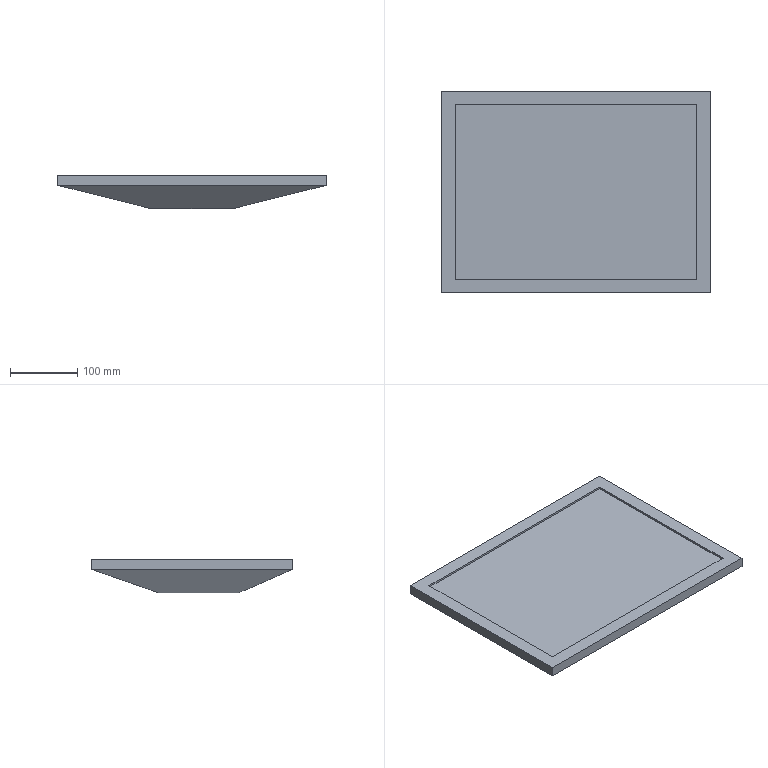Part | SolidWorks | features ICE 2, Extrusion 1, HoleWzd 1 | 1 solid | 31 faces | box 400 x 300 x 50 mm | volume 3576843 mm3 | plane 15 | cylinder 8 | cone 8 | commonest cylinder face diameters 3.3 x8
STEP:
#1=CARTESIAN_POINT('',(50.,398.35,36.8));
#2=VERTEX_POINT('',#1);
#3=CARTESIAN_POINT('',(50.,401.65,36.8));
#4=VERTEX_POINT('',#3);
#5=CARTESIAN_POINT('',(50.,400.,36.8));
#6=DIRECTION('',(0.,0.,-1.));
#7=DIRECTION('',(0.,1.,0.));
#8=AXIS2_PLACEMENT_3D('',#5,#6,#7);
#9=CIRCLE('',#8,1.65);
#10=EDGE_CURVE('',#2,#4,#9,.T.);
#11=ORIENTED_EDGE('',*,*,#10,.F.);
#12=CARTESIAN_POINT('',(50.,398.35,26.7));
#13=VERTEX_POINT('',#12);
#14=CARTESIAN_POINT('',(50.,398.35,26.7));
#15=DIRECTION('',(0.,0.,-1.));
#16=VECTOR('',#15,1000.);
#17=LINE('',#14,#16);
#18=EDGE_CURVE('',#2,#13,#17,.T.);
#19=ORIENTED_EDGE('',*,*,#18,.T.);
#20=CARTESIAN_POINT('',(50.,401.65,26.7));
#21=VERTEX_POINT('',#20);
#22=CARTESIAN_POINT('',(50.,400.,26.7));
#23=DIRECTION('',(0.,0.,-1.));
#24=DIRECTION('',(0.,1.,0.));
#25=AXIS2_PLACEMENT_3D('',#22,#23,#24);
#26=CIRCLE('',#25,1.65);
#27=EDGE_CURVE('',#13,#21,#26,.T.);
#28=ORIENTED_EDGE('',*,*,#27,.T.);
#29=CARTESIAN_POINT('',(50.,401.65,26.7));
#30=DIRECTION('',(0.,0.,-1.));
#31=VECTOR('',#30,1000.);
#32=LINE('',#29,#31);
#33=EDGE_CURVE('',#4,#21,#32,.T.);
#34=ORIENTED_EDGE('',*,*,#33,.F.);
#35=EDGE_LOOP('',(#11,#19,#28,#34));
#36=FACE_OUTER_BOUND('',#35,.T.);
#37=CARTESIAN_POINT('',(50.,400.,26.7));
#38=DIRECTION('',(0.,0.,-1.));
#39=DIRECTION('',(0.,1.,0.));
#40=AXIS2_PLACEMENT_3D('',#37,#38,#39);
#41=CYLINDRICAL_SURFACE('',#40,1.65);
#42=ADVANCED_FACE('',(#36),#41,.F.);
#43=CARTESIAN_POINT('',(50.,400.,37.792));
#44=VERTEX_POINT('',#43);
#45=CARTESIAN_POINT('',(50.,401.65,36.8));
#46=DIRECTION('',(0.,0.8572,-0.515));
#47=VECTOR('',#46,1000.);
#48=LINE('',#45,#47);
#49=EDGE_CURVE('',#44,#4,#48,.T.);
#50=ORIENTED_EDGE('',*,*,#49,.F.);
#51=CARTESIAN_POINT('',(50.,398.35,36.8));
#52=DIRECTION('',(0.,-0.8572,-0.515));
#53=VECTOR('',#52,1000.);
#54=LINE('',#51,#53);
#55=EDGE_CURVE('',#44,#2,#54,.T.);
#56=ORIENTED_EDGE('',*,*,#55,.T.);
#57=ORIENTED_EDGE('',*,*,#10,.T.);
#58=EDGE_LOOP('',(#50,#56,#57));
#59=FACE_OUTER_BOUND('',#58,.T.);
#60=CARTESIAN_POINT('',(50.,400.,36.8));
#61=DIRECTION('',(0.,0.,-1.));
#62=DIRECTION('',(0.,1.,0.));
#63=AXIS2_PLACEMENT_3D('',#60,#61,#62);
#64=CONICAL_SURFACE('',#63,1.65,1.03);
#65=ADVANCED_FACE('',(#59),#64,.F.);
#66=CARTESIAN_POINT('',(-50.,398.35,36.8));
#67=VERTEX_POINT('',#66);
#68=CARTESIAN_POINT('',(-50.,401.65,36.8));
#69=VERTEX_POINT('',#68);
#70=CARTESIAN_POINT('',(-50.,400.,36.8));
#71=DIRECTION('',(0.,0.,-1.));
#72=DIRECTION('',(0.,1.,0.));
#73=AXIS2_PLACEMENT_3D('',#70,#71,#72);
#74=CIRCLE('',#73,1.65);
#75=EDGE_CURVE('',#67,#69,#74,.T.);
#76=ORIENTED_EDGE('',*,*,#75,.F.);
#77=CARTESIAN_POINT('',(-50.,398.35,26.7));
#78=VERTEX_POINT('',#77);
#79=CARTESIAN_POINT('',(-50.,398.35,26.7));
#80=DIRECTION('',(0.,0.,-1.));
#81=VECTOR('',#80,1000.);
#82=LINE('',#79,#81);
#83=EDGE_CURVE('',#67,#78,#82,.T.);
#84=ORIENTED_EDGE('',*,*,#83,.T.);
#85=CARTESIAN_POINT('',(-50.,401.65,26.7));
#86=VERTEX_POINT('',#85);
#87=CARTESIAN_POINT('',(-50.,400.,26.7));
#88=DIRECTION('',(0.,0.,-1.));
#89=DIRECTION('',(0.,1.,0.));
#90=AXIS2_PLACEMENT_3D('',#87,#88,#89);
#91=CIRCLE('',#90,1.65);
#92=EDGE_CURVE('',#78,#86,#91,.T.);
#93=ORIENTED_EDGE('',*,*,#92,.T.);
#94=CARTESIAN_POINT('',(-50.,401.65,26.7));
#95=DIRECTION('',(0.,0.,-1.));
#96=VECTOR('',#95,1000.);
#97=LINE('',#94,#96);
#98=EDGE_CURVE('',#69,#86,#97,.T.);
#99=ORIENTED_EDGE('',*,*,#98,.F.);
#100=EDGE_LOOP('',(#76,#84,#93,#99));
#101=FACE_OUTER_BOUND('',#100,.T.);
#102=CARTESIAN_POINT('',(-50.,400.,26.7));
#103=DIRECTION('',(0.,0.,-1.));
#104=DIRECTION('',(0.,1.,0.));
#105=AXIS2_PLACEMENT_3D('',#102,#103,#104);
#106=CYLINDRICAL_SURFACE('',#105,1.65);
#107=ADVANCED_FACE('',(#101),#106,.F.);
#108=CARTESIAN_POINT('',(-50.,400.,37.792));
#109=VERTEX_POINT('',#108);
#110=CARTESIAN_POINT('',(-50.,401.65,36.8));
#111=DIRECTION('',(0.,0.8572,-0.515));
#112=VECTOR('',#111,1000.);
#113=LINE('',#110,#112);
#114=EDGE_CURVE('',#109,#69,#113,.T.);
#115=ORIENTED_EDGE('',*,*,#114,.F.);
#116=CARTESIAN_POINT('',(-50.,398.35,36.8));
#117=DIRECTION('',(0.,-0.8572,-0.515));
#118=VECTOR('',#117,1000.);
#119=LINE('',#116,#118);
#120=EDGE_CURVE('',#109,#67,#119,.T.);
#121=ORIENTED_EDGE('',*,*,#120,.T.);
#122=ORIENTED_EDGE('',*,*,#75,.T.);
#123=EDGE_LOOP('',(#115,#121,#122));
#124=FACE_OUTER_BOUND('',#123,.T.);
#125=CARTESIAN_POINT('',(-50.,400.,36.8));
#126=DIRECTION('',(0.,0.,-1.));
#127=DIRECTION('',(0.,1.,0.));
#128=AXIS2_PLACEMENT_3D('',#125,#126,#127);
#129=CONICAL_SURFACE('',#128,1.65,1.03);
#130=ADVANCED_FACE('',(#124),#129,.F.);
#131=CARTESIAN_POINT('',(-50.,298.35,36.8));
#132=VERTEX_POINT('',#131);
#133=CARTESIAN_POINT('',(-50.,301.65,36.8));
#134=VERTEX_POINT('',#133);
#135=CARTESIAN_POINT('',(-50.,300.,36.8));
#136=DIRECTION('',(0.,0.,-1.));
#137=DIRECTION('',(0.,1.,0.));
#138=AXIS2_PLACEMENT_3D('',#135,#136,#137);
#139=CIRCLE('',#138,1.65);
#140=EDGE_CURVE('',#132,#134,#139,.T.);
#141=ORIENTED_EDGE('',*,*,#140,.F.);
#142=CARTESIAN_POINT('',(-50.,298.35,26.7));
#143=VERTEX_POINT('',#142);
#144=CARTESIAN_POINT('',(-50.,298.35,26.7));
#145=DIRECTION('',(0.,0.,-1.));
#146=VECTOR('',#145,1000.);
#147=LINE('',#144,#146);
#148=EDGE_CURVE('',#132,#143,#147,.T.);
#149=ORIENTED_EDGE('',*,*,#148,.T.);
#150=CARTESIAN_POINT('',(-50.,301.65,26.7));
#151=VERTEX_POINT('',#150);
#152=CARTESIAN_POINT('',(-50.,300.,26.7));
#153=DIRECTION('',(0.,0.,-1.));
#154=DIRECTION('',(0.,1.,0.));
#155=AXIS2_PLACEMENT_3D('',#152,#153,#154);
#156=CIRCLE('',#155,1.65);
#157=EDGE_CURVE('',#143,#151,#156,.T.);
#158=ORIENTED_EDGE('',*,*,#157,.T.);
#159=CARTESIAN_POINT('',(-50.,301.65,26.7));
#160=DIRECTION('',(0.,0.,-1.));
#161=VECTOR('',#160,1000.);
#162=LINE('',#159,#161);
#163=EDGE_CURVE('',#134,#151,#162,.T.);
#164=ORIENTED_EDGE('',*,*,#163,.F.);
#165=EDGE_LOOP('',(#141,#149,#158,#164));
#166=FACE_OUTER_BOUND('',#165,.T.);
#167=CARTESIAN_POINT('',(-50.,300.,26.7));
#168=DIRECTION('',(0.,0.,-1.));
#169=DIRECTION('',(0.,1.,0.));
#170=AXIS2_PLACEMENT_3D('',#167,#168,#169);
#171=CYLINDRICAL_SURFACE('',#170,1.65);
#172=ADVANCED_FACE('',(#166),#171,.F.);
#173=CARTESIAN_POINT('',(-50.,300.,37.792));
#174=VERTEX_POINT('',#173);
#175=CARTESIAN_POINT('',(-50.,301.65,36.8));
#176=DIRECTION('',(0.,0.8572,-0.515));
#177=VECTOR('',#176,1000.);
#178=LINE('',#175,#177);
#179=EDGE_CURVE('',#174,#134,#178,.T.);
#180=ORIENTED_EDGE('',*,*,#179,.F.);
#181=CARTESIAN_POINT('',(-50.,298.35,36.8));
#182=DIRECTION('',(0.,-0.8572,-0.515));
#183=VECTOR('',#182,1000.);
#184=LINE('',#181,#183);
#185=EDGE_CURVE('',#174,#132,#184,.T.);
#186=ORIENTED_EDGE('',*,*,#185,.T.);
#187=ORIENTED_EDGE('',*,*,#140,.T.);
#188=EDGE_LOOP('',(#180,#186,#187));
#189=FACE_OUTER_BOUND('',#188,.T.);
#190=CARTESIAN_POINT('',(-50.,300.,36.8));
#191=DIRECTION('',(0.,0.,-1.));
#192=DIRECTION('',(0.,1.,0.));
#193=AXIS2_PLACEMENT_3D('',#190,#191,#192);
#194=CONICAL_SURFACE('',#193,1.65,1.03);
#195=ADVANCED_FACE('',(#189),#194,.F.);
#196=CARTESIAN_POINT('',(50.,298.35,36.8));
#197=VERTEX_POINT('',#196);
#198=CARTESIAN_POINT('',(50.,301.65,36.8));
#199=VERTEX_POINT('',#198);
#200=CARTESIAN_POINT('',(50.,300.,36.8));
#201=DIRECTION('',(0.,0.,-1.));
#202=DIRECTION('',(0.,1.,0.));
#203=AXIS2_PLACEMENT_3D('',#200,#201,#202);
#204=CIRCLE('',#203,1.65);
#205=EDGE_CURVE('',#197,#199,#204,.T.);
#206=ORIENTED_EDGE('',*,*,#205,.F.);
#207=CARTESIAN_POINT('',(50.,298.35,26.7));
#208=VERTEX_POINT('',#207);
#209=CARTESIAN_POINT('',(50.,298.35,26.7));
#210=DIRECTION('',(0.,0.,-1.));
#211=VECTOR('',#210,1000.);
#212=LINE('',#209,#211);
#213=EDGE_CURVE('',#197,#208,#212,.T.);
#214=ORIENTED_EDGE('',*,*,#213,.T.);
#215=CARTESIAN_POINT('',(50.,301.65,26.7));
#216=VERTEX_POINT('',#215);
#217=CARTESIAN_POINT('',(50.,300.,26.7));
#218=DIRECTION('',(0.,0.,-1.));
#219=DIRECTION('',(0.,1.,0.));
#220=AXIS2_PLACEMENT_3D('',#217,#218,#219);
#221=CIRCLE('',#220,1.65);
#222=EDGE_CURVE('',#208,#216,#221,.T.);
#223=ORIENTED_EDGE('',*,*,#222,.T.);
#224=CARTESIAN_POINT('',(50.,301.65,26.7));
#225=DIRECTION('',(0.,0.,-1.));
#226=VECTOR('',#225,1000.);
#227=LINE('',#224,#226);
#228=EDGE_CURVE('',#199,#216,#227,.T.);
#229=ORIENTED_EDGE('',*,*,#228,.F.);
#230=EDGE_LOOP('',(#206,#214,#223,#229));
#231=FACE_OUTER_BOUND('',#230,.T.);
#232=CARTESIAN_POINT('',(50.,300.,26.7));
#233=DIRECTION('',(0.,0.,-1.));
#234=DIRECTION('',(0.,1.,0.));
#235=AXIS2_PLACEMENT_3D('',#232,#233,#234);
#236=CYLINDRICAL_SURFACE('',#235,1.65);
#237=ADVANCED_FACE('',(#231),#236,.F.);
#238=CARTESIAN_POINT('',(50.,300.,37.792));
#239=VERTEX_POINT('',#238);
#240=CARTESIAN_POINT('',(50.,301.65,36.8));
#241=DIRECTION('',(0.,0.8572,-0.515));
#242=VECTOR('',#241,1000.);
#243=LINE('',#240,#242);
#244=EDGE_CURVE('',#239,#199,#243,.T.);
#245=ORIENTED_EDGE('',*,*,#244,.F.);
#246=CARTESIAN_POINT('',(50.,298.35,36.8));
#247=DIRECTION('',(0.,-0.8572,-0.515));
#248=VECTOR('',#247,1000.);
#249=LINE('',#246,#248);
#250=EDGE_CURVE('',#239,#197,#249,.T.);
#251=ORIENTED_EDGE('',*,*,#250,.T.);
#252=ORIENTED_EDGE('',*,*,#205,.T.);
#253=EDGE_LOOP('',(#245,#251,#252));
#254=FACE_OUTER_BOUND('',#253,.T.);
#255=CARTESIAN_POINT('',(50.,300.,36.8));
#256=DIRECTION('',(0.,0.,-1.));
#257=DIRECTION('',(0.,1.,0.));
#258=AXIS2_PLACEMENT_3D('',#255,#256,#257);
#259=CONICAL_SURFACE('',#258,1.65,1.03);
#260=ADVANCED_FACE('',(#254),#259,.F.);
#261=CARTESIAN_POINT('',(50.,400.,26.7));
#262=DIRECTION('',(0.,0.,-1.));
#263=DIRECTION('',(0.,1.,0.));
#264=AXIS2_PLACEMENT_3D('',#261,#262,#263);
#265=CIRCLE('',#264,1.65);
#266=EDGE_CURVE('',#21,#13,#265,.T.);
#267=ORIENTED_EDGE('',*,*,#266,.F.);
#268=ORIENTED_EDGE('',*,*,#27,.F.);
#269=EDGE_LOOP('',(#267,#268));
#270=FACE_BOUND('',#269,.T.);
#271=CARTESIAN_POINT('',(-50.,400.,26.7));
#272=DIRECTION('',(0.,0.,-1.));
#273=DIRECTION('',(0.,1.,0.));
#274=AXIS2_PLACEMENT_3D('',#271,#272,#273);
#275=CIRCLE('',#274,1.65);
#276=EDGE_CURVE('',#86,#78,#275,.T.);
#277=ORIENTED_EDGE('',*,*,#276,.F.);
#278=ORIENTED_EDGE('',*,*,#92,.F.);
#279=EDGE_LOOP('',(#277,#278));
#280=FACE_BOUND('',#279,.T.);
#281=CARTESIAN_POINT('',(-50.,300.,26.7));
#282=DIRECTION('',(0.,0.,-1.));
#283=DIRECTION('',(0.,1.,0.));
#284=AXIS2_PLACEMENT_3D('',#281,#282,#283);
#285=CIRCLE('',#284,1.65);
#286=EDGE_CURVE('',#151,#143,#285,.T.);
#287=ORIENTED_EDGE('',*,*,#286,.F.);
#288=ORIENTED_EDGE('',*,*,#157,.F.);
#289=EDGE_LOOP('',(#287,#288));
#290=FACE_BOUND('',#289,.T.);
#291=CARTESIAN_POINT('',(50.,300.,26.7));
#292=DIRECTION('',(0.,0.,-1.));
#293=DIRECTION('',(0.,1.,0.));
#294=AXIS2_PLACEMENT_3D('',#291,#292,#293);
#295=CIRCLE('',#294,1.65);
#296=EDGE_CURVE('',#216,#208,#295,.T.);
#297=ORIENTED_EDGE('',*,*,#296,.F.);
#298=ORIENTED_EDGE('',*,*,#222,.F.);
#299=EDGE_LOOP('',(#297,#298));
#300=FACE_BOUND('',#299,.T.);
#301=CARTESIAN_POINT('',(60.,290.,26.7));
#302=VERTEX_POINT('',#301);
#303=CARTESIAN_POINT('',(60.,410.,26.7));
#304=VERTEX_POINT('',#303);
#305=CARTESIAN_POINT('',(60.,209.999,26.7));
#306=DIRECTION('',(0.,1.,0.));
#307=VECTOR('',#306,1000.);
#308=LINE('',#305,#307);
#309=EDGE_CURVE('',#302,#304,#308,.T.);
#310=ORIENTED_EDGE('',*,*,#309,.F.);
#311=CARTESIAN_POINT('',(-60.,290.,26.7));
#312=VERTEX_POINT('',#311);
#313=CARTESIAN_POINT('',(200.,290.,26.7));
#314=DIRECTION('',(-1.,0.,0.));
#315=VECTOR('',#314,1000.);
#316=LINE('',#313,#315);
#317=EDGE_CURVE('',#302,#312,#316,.T.);
#318=ORIENTED_EDGE('',*,*,#317,.T.);
#319=CARTESIAN_POINT('',(-60.,410.,26.7));
#320=VERTEX_POINT('',#319);
#321=CARTESIAN_POINT('',(-60.,209.999,26.7));
#322=DIRECTION('',(0.,1.,0.));
#323=VECTOR('',#322,1000.);
#324=LINE('',#321,#323);
#325=EDGE_CURVE('',#312,#320,#324,.T.);
#326=ORIENTED_EDGE('',*,*,#325,.T.);
#327=CARTESIAN_POINT('',(200.,410.,26.7));
#328=DIRECTION('',(-1.,0.,0.));
#329=VECTOR('',#328,1000.);
#330=LINE('',#327,#329);
#331=EDGE_CURVE('',#304,#320,#330,.T.);
#332=ORIENTED_EDGE('',*,*,#331,.F.);
#333=EDGE_LOOP('',(#310,#318,#326,#332));
#334=FACE_OUTER_BOUND('',#333,.T.);
#335=CARTESIAN_POINT('',(200.,410.,26.7));
#336=DIRECTION('',(0.,0.,-1.));
#337=DIRECTION('',(0.,1.,0.));
#338=AXIS2_PLACEMENT_3D('',#335,#336,#337);
#339=PLANE('',#338);
#340=ADVANCED_FACE('',(#270,#280,#290,#300,#334),#339,.T.);
#341=CARTESIAN_POINT('',(200.,510.,61.7));
#342=VERTEX_POINT('',#341);
#343=CARTESIAN_POINT('',(63.747,412.676,27.637));
#344=DIRECTION('',(-0.7974,-0.5696,-0.1994));
#345=VECTOR('',#344,1000.);
#346=LINE('',#343,#345);
#347=EDGE_CURVE('',#342,#304,#346,.T.);
#348=ORIENTED_EDGE('',*,*,#347,.T.);
#349=ORIENTED_EDGE('',*,*,#331,.T.);
#350=CARTESIAN_POINT('',(-200.,510.,61.7));
#351=VERTEX_POINT('',#350);
#352=CARTESIAN_POINT('',(30.836,345.117,3.991));
#353=DIRECTION('',(-0.7974,0.5696,0.1994));
#354=VECTOR('',#353,1000.);
#355=LINE('',#352,#354);
#356=EDGE_CURVE('',#320,#351,#355,.T.);
#357=ORIENTED_EDGE('',*,*,#356,.T.);
#358=CARTESIAN_POINT('',(200.,510.,61.7));
#359=DIRECTION('',(-1.,0.,0.));
#360=VECTOR('',#359,1000.);
#361=LINE('',#358,#360);
#362=EDGE_CURVE('',#342,#351,#361,.T.);
#363=ORIENTED_EDGE('',*,*,#362,.F.);
#364=EDGE_LOOP('',(#348,#349,#357,#363));
#365=FACE_OUTER_BOUND('',#364,.T.);
#366=CARTESIAN_POINT('',(200.,410.,26.7));
#367=DIRECTION('',(0.,0.3304,-0.9439));
#368=DIRECTION('',(0.,0.9439,0.3304));
#369=AXIS2_PLACEMENT_3D('',#366,#367,#368);
#370=PLANE('',#369);
#371=ADVANCED_FACE('',(#365),#370,.T.);
#372=ORIENTED_EDGE('',*,*,#362,.T.);
#373=CARTESIAN_POINT('',(-200.,510.,76.7));
#374=VERTEX_POINT('',#373);
#375=CARTESIAN_POINT('',(-200.,510.,61.7));
#376=DIRECTION('',(0.,0.,-1.));
#377=VECTOR('',#376,1000.);
#378=LINE('',#375,#377);
#379=EDGE_CURVE('',#374,#351,#378,.T.);
#380=ORIENTED_EDGE('',*,*,#379,.F.);
#381=CARTESIAN_POINT('',(200.,510.,76.7));
#382=VERTEX_POINT('',#381);
#383=CARTESIAN_POINT('',(200.,510.,76.7));
#384=DIRECTION('',(-1.,0.,0.));
#385=VECTOR('',#384,1000.);
#386=LINE('',#383,#385);
#387=EDGE_CURVE('',#382,#374,#386,.T.);
#388=ORIENTED_EDGE('',*,*,#387,.F.);
#389=CARTESIAN_POINT('',(200.,510.,61.7));
#390=DIRECTION('',(0.,0.,-1.));
#391=VECTOR('',#390,1000.);
#392=LINE('',#389,#391);
#393=EDGE_CURVE('',#382,#342,#392,.T.);
#394=ORIENTED_EDGE('',*,*,#393,.T.);
#395=EDGE_LOOP('',(#372,#380,#388,#394));
#396=FACE_OUTER_BOUND('',#395,.T.);
#397=CARTESIAN_POINT('',(200.,510.,61.7));
#398=DIRECTION('',(0.,1.,0.));
#399=DIRECTION('',(0.,0.,1.));
#400=AXIS2_PLACEMENT_3D('',#397,#398,#399);
#401=PLANE('',#400);
#402=ADVANCED_FACE('',(#396),#401,.T.);
#403=CARTESIAN_POINT('',(180.,230.,76.7));
#404=VERTEX_POINT('',#403);
#405=CARTESIAN_POINT('',(180.,490.,76.7));
#406=VERTEX_POINT('',#405);
#407=CARTESIAN_POINT('',(180.,230.,76.7));
#408=DIRECTION('',(0.,1.,0.));
#409=VECTOR('',#408,1000.);
#410=LINE('',#407,#409);
#411=EDGE_CURVE('',#404,#406,#410,.T.);
#412=ORIENTED_EDGE('',*,*,#411,.F.);
#413=CARTESIAN_POINT('',(-180.,230.,76.7));
#414=VERTEX_POINT('',#413);
#415=CARTESIAN_POINT('',(-180.,230.,76.7));
#416=DIRECTION('',(1.,0.,0.));
#417=VECTOR('',#416,1000.);
#418=LINE('',#415,#417);
#419=EDGE_CURVE('',#414,#404,#418,.T.);
#420=ORIENTED_EDGE('',*,*,#419,.F.);
#421=CARTESIAN_POINT('',(-180.,490.,76.7));
#422=VERTEX_POINT('',#421);
#423=CARTESIAN_POINT('',(-180.,490.,76.7));
#424=DIRECTION('',(0.,-1.,0.));
#425=VECTOR('',#424,1000.);
#426=LINE('',#423,#425);
#427=EDGE_CURVE('',#422,#414,#426,.T.);
#428=ORIENTED_EDGE('',*,*,#427,.F.);
#429=CARTESIAN_POINT('',(180.,490.,76.7));
#430=DIRECTION('',(-1.,0.,0.));
#431=VECTOR('',#430,1000.);
#432=LINE('',#429,#431);
#433=EDGE_CURVE('',#406,#422,#432,.T.);
#434=ORIENTED_EDGE('',*,*,#433,.F.);
#435=EDGE_LOOP('',(#412,#420,#428,#434));
#436=FACE_BOUND('',#435,.T.);
#437=ORIENTED_EDGE('',*,*,#387,.T.);
#438=CARTESIAN_POINT('',(-200.,210.,76.7));
#439=VERTEX_POINT('',#438);
#440=CARTESIAN_POINT('',(-200.,510.,76.7));
#441=DIRECTION('',(0.,1.,0.));
#442=VECTOR('',#441,1000.);
#443=LINE('',#440,#442);
#444=EDGE_CURVE('',#439,#374,#443,.T.);
#445=ORIENTED_EDGE('',*,*,#444,.F.);
#446=CARTESIAN_POINT('',(200.,210.,76.7));
#447=VERTEX_POINT('',#446);
#448=CARTESIAN_POINT('',(200.,210.,76.7));
#449=DIRECTION('',(-1.,0.,0.));
#450=VECTOR('',#449,1000.);
#451=LINE('',#448,#450);
#452=EDGE_CURVE('',#447,#439,#451,.T.);
#453=ORIENTED_EDGE('',*,*,#452,.F.);
#454=CARTESIAN_POINT('',(200.,510.,76.7));
#455=DIRECTION('',(0.,1.,0.));
#456=VECTOR('',#455,1000.);
#457=LINE('',#454,#456);
#458=EDGE_CURVE('',#447,#382,#457,.T.);
#459=ORIENTED_EDGE('',*,*,#458,.T.);
#460=EDGE_LOOP('',(#437,#445,#453,#459));
#461=FACE_OUTER_BOUND('',#460,.T.);
#462=CARTESIAN_POINT('',(200.,510.,76.7));
#463=DIRECTION('',(0.,0.,1.));
#464=DIRECTION('',(0.,-1.,0.));
#465=AXIS2_PLACEMENT_3D('',#462,#463,#464);
#466=PLANE('',#465);
#467=ADVANCED_FACE('',(#436,#461),#466,.T.);
#468=ORIENTED_EDGE('',*,*,#452,.T.);
#469=CARTESIAN_POINT('',(-200.,210.,61.7));
#470=VERTEX_POINT('',#469);
#471=CARTESIAN_POINT('',(-200.,210.,76.7));
#472=DIRECTION('',(0.,0.,1.));
#473=VECTOR('',#472,1000.);
#474=LINE('',#471,#473);
#475=EDGE_CURVE('',#470,#439,#474,.T.);
#476=ORIENTED_EDGE('',*,*,#475,.F.);
#477=CARTESIAN_POINT('',(200.,210.,61.7));
#478=VERTEX_POINT('',#477);
#479=CARTESIAN_POINT('',(200.,210.,61.7));
#480=DIRECTION('',(-1.,0.,0.));
#481=VECTOR('',#480,1000.);
#482=LINE('',#479,#481);
#483=EDGE_CURVE('',#478,#470,#482,.T.);
#484=ORIENTED_EDGE('',*,*,#483,.F.);
#485=CARTESIAN_POINT('',(200.,210.,76.7));
#486=DIRECTION('',(0.,0.,1.));
#487=VECTOR('',#486,1000.);
#488=LINE('',#485,#487);
#489=EDGE_CURVE('',#478,#447,#488,.T.);
#490=ORIENTED_EDGE('',*,*,#489,.T.);
#491=EDGE_LOOP('',(#468,#476,#484,#490));
#492=FACE_OUTER_BOUND('',#491,.T.);
#493=CARTESIAN_POINT('',(200.,210.,76.7));
#494=DIRECTION('',(0.,-1.,0.));
#495=DIRECTION('',(0.,0.,-1.));
#496=AXIS2_PLACEMENT_3D('',#493,#494,#495);
#497=PLANE('',#496);
#498=ADVANCED_FACE('',(#492),#497,.T.);
#499=CARTESIAN_POINT('',(200.,210.,61.7));
#500=DIRECTION('',(0.8485,-0.4848,0.2121));
#501=VECTOR('',#500,1000.);
#502=LINE('',#499,#501);
#503=EDGE_CURVE('',#302,#478,#502,.T.);
#504=ORIENTED_EDGE('',*,*,#503,.T.);
#505=ORIENTED_EDGE('',*,*,#483,.T.);
#506=CARTESIAN_POINT('',(-92.911,271.194,34.928));
#507=DIRECTION('',(0.8485,0.4848,-0.2121));
#508=VECTOR('',#507,1000.);
#509=LINE('',#506,#508);
#510=EDGE_CURVE('',#470,#312,#509,.T.);
#511=ORIENTED_EDGE('',*,*,#510,.T.);
#512=ORIENTED_EDGE('',*,*,#317,.F.);
#513=EDGE_LOOP('',(#504,#505,#511,#512));
#514=FACE_OUTER_BOUND('',#513,.T.);
#515=CARTESIAN_POINT('',(200.,290.,26.7));
#516=DIRECTION('',(0.,-0.4008,-0.9162));
#517=DIRECTION('',(0.,0.9162,-0.4008));
#518=AXIS2_PLACEMENT_3D('',#515,#516,#517);
#519=PLANE('',#518);
#520=ADVANCED_FACE('',(#514),#519,.T.);
#521=CARTESIAN_POINT('',(200.,209.999,61.7));
#522=DIRECTION('',(0.,1.,0.));
#523=VECTOR('',#522,1000.);
#524=LINE('',#521,#523);
#525=EDGE_CURVE('',#478,#342,#524,.T.);
#526=ORIENTED_EDGE('',*,*,#525,.T.);
#527=ORIENTED_EDGE('',*,*,#393,.F.);
#528=ORIENTED_EDGE('',*,*,#458,.F.);
#529=ORIENTED_EDGE('',*,*,#489,.F.);
#530=EDGE_LOOP('',(#526,#527,#528,#529));
#531=FACE_OUTER_BOUND('',#530,.T.);
#532=CARTESIAN_POINT('',(200.,0.,0.));
#533=DIRECTION('',(1.,0.,0.));
#534=DIRECTION('',(0.,0.,-1.));
#535=AXIS2_PLACEMENT_3D('',#532,#533,#534);
#536=PLANE('',#535);
#537=ADVANCED_FACE('',(#531),#536,.T.);
#538=ORIENTED_EDGE('',*,*,#379,.T.);
#539=CARTESIAN_POINT('',(-200.,209.999,61.7));
#540=DIRECTION('',(0.,1.,0.));
#541=VECTOR('',#540,1000.);
#542=LINE('',#539,#541);
#543=EDGE_CURVE('',#470,#351,#542,.T.);
#544=ORIENTED_EDGE('',*,*,#543,.F.);
#545=ORIENTED_EDGE('',*,*,#475,.T.);
#546=ORIENTED_EDGE('',*,*,#444,.T.);
#547=EDGE_LOOP('',(#538,#544,#545,#546));
#548=FACE_OUTER_BOUND('',#547,.T.);
#549=CARTESIAN_POINT('',(-200.,0.,0.));
#550=DIRECTION('',(1.,0.,0.));
#551=DIRECTION('',(0.,0.,-1.));
#552=AXIS2_PLACEMENT_3D('',#549,#550,#551);
#553=PLANE('',#552);
#554=ADVANCED_FACE('',(#548),#553,.F.);
#555=ORIENTED_EDGE('',*,*,#411,.T.);
#556=CARTESIAN_POINT('',(180.,490.,73.7));
#557=VERTEX_POINT('',#556);
#558=CARTESIAN_POINT('',(180.,490.,73.7));
#559=DIRECTION('',(0.,0.,1.));
#560=VECTOR('',#559,1000.);
#561=LINE('',#558,#560);
#562=EDGE_CURVE('',#557,#406,#561,.T.);
#563=ORIENTED_EDGE('',*,*,#562,.F.);
#564=CARTESIAN_POINT('',(180.,230.,73.7));
#565=VERTEX_POINT('',#564);
#566=CARTESIAN_POINT('',(180.,230.,73.7));
#567=DIRECTION('',(0.,1.,0.));
#568=VECTOR('',#567,1000.);
#569=LINE('',#566,#568);
#570=EDGE_CURVE('',#565,#557,#569,.T.);
#571=ORIENTED_EDGE('',*,*,#570,.F.);
#572=CARTESIAN_POINT('',(180.,230.,73.7));
#573=DIRECTION('',(0.,0.,1.));
#574=VECTOR('',#573,1000.);
#575=LINE('',#572,#574);
#576=EDGE_CURVE('',#565,#404,#575,.T.);
#577=ORIENTED_EDGE('',*,*,#576,.T.);
#578=EDGE_LOOP('',(#555,#563,#571,#577));
#579=FACE_OUTER_BOUND('',#578,.T.);
#580=CARTESIAN_POINT('',(180.,230.,73.7));
#581=DIRECTION('',(1.,0.,0.));
#582=DIRECTION('',(0.,0.,-1.));
#583=AXIS2_PLACEMENT_3D('',#580,#581,#582);
#584=PLANE('',#583);
#585=ADVANCED_FACE('',(#579),#584,.F.);
#586=ORIENTED_EDGE('',*,*,#419,.T.);
#587=ORIENTED_EDGE('',*,*,#576,.F.);
#588=CARTESIAN_POINT('',(-180.,230.,73.7));
#589=VERTEX_POINT('',#588);
#590=CARTESIAN_POINT('',(-180.,230.,73.7));
#591=DIRECTION('',(1.,0.,0.));
#592=VECTOR('',#591,1000.);
#593=LINE('',#590,#592);
#594=EDGE_CURVE('',#589,#565,#593,.T.);
#595=ORIENTED_EDGE('',*,*,#594,.F.);
#596=CARTESIAN_POINT('',(-180.,230.,73.7));
#597=DIRECTION('',(0.,0.,1.));
#598=VECTOR('',#597,1000.);
#599=LINE('',#596,#598);
#600=EDGE_CURVE('',#589,#414,#599,.T.);
#601=ORIENTED_EDGE('',*,*,#600,.T.);
#602=EDGE_LOOP('',(#586,#587,#595,#601));
#603=FACE_OUTER_BOUND('',#602,.T.);
#604=CARTESIAN_POINT('',(-180.,230.,73.7));
#605=DIRECTION('',(0.,-1.,0.));
#606=DIRECTION('',(0.,0.,-1.));
#607=AXIS2_PLACEMENT_3D('',#604,#605,#606);
#608=PLANE('',#607);
#609=ADVANCED_FACE('',(#603),#608,.F.);
#610=ORIENTED_EDGE('',*,*,#427,.T.);
#611=ORIENTED_EDGE('',*,*,#600,.F.);
#612=CARTESIAN_POINT('',(-180.,490.,73.7));
#613=VERTEX_POINT('',#612);
#614=CARTESIAN_POINT('',(-180.,490.,73.7));
#615=DIRECTION('',(0.,-1.,0.));
#616=VECTOR('',#615,1000.);
#617=LINE('',#614,#616);
#618=EDGE_CURVE('',#613,#589,#617,.T.);
#619=ORIENTED_EDGE('',*,*,#618,.F.);
#620=CARTESIAN_POINT('',(-180.,490.,73.7));
#621=DIRECTION('',(0.,0.,1.));
#622=VECTOR('',#621,1000.);
#623=LINE('',#620,#622);
#624=EDGE_CURVE('',#613,#422,#623,.T.);
#625=ORIENTED_EDGE('',*,*,#624,.T.);
#626=EDGE_LOOP('',(#610,#611,#619,#625));
#627=FACE_OUTER_BOUND('',#626,.T.);
#628=CARTESIAN_POINT('',(-180.,490.,73.7));
#629=DIRECTION('',(-1.,0.,0.));
#630=DIRECTION('',(0.,0.,1.));
#631=AXIS2_PLACEMENT_3D('',#628,#629,#630);
#632=PLANE('',#631);
#633=ADVANCED_FACE('',(#627),#632,.F.);
#634=ORIENTED_EDGE('',*,*,#433,.T.);
#635=ORIENTED_EDGE('',*,*,#624,.F.);
#636=CARTESIAN_POINT('',(180.,490.,73.7));
#637=DIRECTION('',(-1.,0.,0.));
#638=VECTOR('',#637,1000.);
#639=LINE('',#636,#638);
#640=EDGE_CURVE('',#557,#613,#639,.T.);
#641=ORIENTED_EDGE('',*,*,#640,.F.);
#642=ORIENTED_EDGE('',*,*,#562,.T.);
#643=EDGE_LOOP('',(#634,#635,#641,#642));
#644=FACE_OUTER_BOUND('',#643,.T.);
#645=CARTESIAN_POINT('',(180.,490.,73.7));
#646=DIRECTION('',(0.,1.,0.));
#647=DIRECTION('',(0.,0.,1.));
#648=AXIS2_PLACEMENT_3D('',#645,#646,#647);
#649=PLANE('',#648);
#650=ADVANCED_FACE('',(#644),#649,.F.);
#651=ORIENTED_EDGE('',*,*,#570,.T.);
#652=ORIENTED_EDGE('',*,*,#640,.T.);
#653=ORIENTED_EDGE('',*,*,#618,.T.);
#654=ORIENTED_EDGE('',*,*,#594,.T.);
#655=EDGE_LOOP('',(#651,#652,#653,#654));
#656=FACE_OUTER_BOUND('',#655,.T.);
#657=CARTESIAN_POINT('',(0.,0.,73.7));
#658=DIRECTION('',(0.,0.,1.));
#659=DIRECTION('',(1.,0.,0.));
#660=AXIS2_PLACEMENT_3D('',#657,#658,#659);
#661=PLANE('',#660);
#662=ADVANCED_FACE('',(#656),#661,.T.);
#663=ORIENTED_EDGE('',*,*,#325,.F.);
#664=ORIENTED_EDGE('',*,*,#510,.F.);
#665=ORIENTED_EDGE('',*,*,#543,.T.);
#666=ORIENTED_EDGE('',*,*,#356,.F.);
#667=EDGE_LOOP('',(#663,#664,#665,#666));
#668=FACE_OUTER_BOUND('',#667,.T.);
#669=CARTESIAN_POINT('',(-60.,209.999,26.7));
#670=DIRECTION('',(0.2425,0.,0.9701));
#671=DIRECTION('',(0.9701,0.,-0.2425));
#672=AXIS2_PLACEMENT_3D('',#669,#670,#671);
#673=PLANE('',#672);
#674=ADVANCED_FACE('',(#668),#673,.F.);
#675=ORIENTED_EDGE('',*,*,#525,.F.);
#676=ORIENTED_EDGE('',*,*,#503,.F.);
#677=ORIENTED_EDGE('',*,*,#309,.T.);
#678=ORIENTED_EDGE('',*,*,#347,.F.);
#679=EDGE_LOOP('',(#675,#676,#677,#678));
#680=FACE_OUTER_BOUND('',#679,.T.);
#681=CARTESIAN_POINT('',(200.,209.999,61.7));
#682=DIRECTION('',(-0.2425,0.,0.9701));
#683=DIRECTION('',(0.9701,0.,0.2425));
#684=AXIS2_PLACEMENT_3D('',#681,#682,#683);
#685=PLANE('',#684);
#686=ADVANCED_FACE('',(#680),#685,.F.);
#687=ORIENTED_EDGE('',*,*,#250,.F.);
#688=ORIENTED_EDGE('',*,*,#244,.T.);
#689=CARTESIAN_POINT('',(50.,300.,36.8));
#690=DIRECTION('',(0.,0.,-1.));
#691=DIRECTION('',(0.,1.,0.));
#692=AXIS2_PLACEMENT_3D('',#689,#690,#691);
#693=CIRCLE('',#692,1.65);
#694=EDGE_CURVE('',#199,#197,#693,.T.);
#695=ORIENTED_EDGE('',*,*,#694,.T.);
#696=EDGE_LOOP('',(#687,#688,#695));
#697=FACE_OUTER_BOUND('',#696,.T.);
#698=CARTESIAN_POINT('',(50.,300.,36.8));
#699=DIRECTION('',(0.,0.,-1.));
#700=DIRECTION('',(0.,1.,0.));
#701=AXIS2_PLACEMENT_3D('',#698,#699,#700);
#702=CONICAL_SURFACE('',#701,1.65,1.03);
#703=ADVANCED_FACE('',(#697),#702,.F.);
#704=ORIENTED_EDGE('',*,*,#213,.F.);
#705=ORIENTED_EDGE('',*,*,#694,.F.);
#706=ORIENTED_EDGE('',*,*,#228,.T.);
#707=ORIENTED_EDGE('',*,*,#296,.T.);
#708=EDGE_LOOP('',(#704,#705,#706,#707));
#709=FACE_OUTER_BOUND('',#708,.T.);
#710=CARTESIAN_POINT('',(50.,300.,26.7));
#711=DIRECTION('',(0.,0.,-1.));
#712=DIRECTION('',(0.,1.,0.));
#713=AXIS2_PLACEMENT_3D('',#710,#711,#712);
#714=CYLINDRICAL_SURFACE('',#713,1.65);
#715=ADVANCED_FACE('',(#709),#714,.F.);
#716=ORIENTED_EDGE('',*,*,#185,.F.);
#717=ORIENTED_EDGE('',*,*,#179,.T.);
#718=CARTESIAN_POINT('',(-50.,300.,36.8));
#719=DIRECTION('',(0.,0.,-1.));
#720=DIRECTION('',(0.,1.,0.));
#721=AXIS2_PLACEMENT_3D('',#718,#719,#720);
#722=CIRCLE('',#721,1.65);
#723=EDGE_CURVE('',#134,#132,#722,.T.);
#724=ORIENTED_EDGE('',*,*,#723,.T.);
#725=EDGE_LOOP('',(#716,#717,#724));
#726=FACE_OUTER_BOUND('',#725,.T.);
#727=CARTESIAN_POINT('',(-50.,300.,36.8));
#728=DIRECTION('',(0.,0.,-1.));
#729=DIRECTION('',(0.,1.,0.));
#730=AXIS2_PLACEMENT_3D('',#727,#728,#729);
#731=CONICAL_SURFACE('',#730,1.65,1.03);
#732=ADVANCED_FACE('',(#726),#731,.F.);
#733=ORIENTED_EDGE('',*,*,#148,.F.);
#734=ORIENTED_EDGE('',*,*,#723,.F.);
#735=ORIENTED_EDGE('',*,*,#163,.T.);
#736=ORIENTED_EDGE('',*,*,#286,.T.);
#737=EDGE_LOOP('',(#733,#734,#735,#736));
#738=FACE_OUTER_BOUND('',#737,.T.);
#739=CARTESIAN_POINT('',(-50.,300.,26.7));
#740=DIRECTION('',(0.,0.,-1.));
#741=DIRECTION('',(0.,1.,0.));
#742=AXIS2_PLACEMENT_3D('',#739,#740,#741);
#743=CYLINDRICAL_SURFACE('',#742,1.65);
#744=ADVANCED_FACE('',(#738),#743,.F.);
#745=ORIENTED_EDGE('',*,*,#120,.F.);
#746=ORIENTED_EDGE('',*,*,#114,.T.);
#747=CARTESIAN_POINT('',(-50.,400.,36.8));
#748=DIRECTION('',(0.,0.,-1.));
#749=DIRECTION('',(0.,1.,0.));
#750=AXIS2_PLACEMENT_3D('',#747,#748,#749);
#751=CIRCLE('',#750,1.65);
#752=EDGE_CURVE('',#69,#67,#751,.T.);
#753=ORIENTED_EDGE('',*,*,#752,.T.);
#754=EDGE_LOOP('',(#745,#746,#753));
#755=FACE_OUTER_BOUND('',#754,.T.);
#756=CARTESIAN_POINT('',(-50.,400.,36.8));
#757=DIRECTION('',(0.,0.,-1.));
#758=DIRECTION('',(0.,1.,0.));
#759=AXIS2_PLACEMENT_3D('',#756,#757,#758);
#760=CONICAL_SURFACE('',#759,1.65,1.03);
#761=ADVANCED_FACE('',(#755),#760,.F.);
#762=ORIENTED_EDGE('',*,*,#83,.F.);
#763=ORIENTED_EDGE('',*,*,#752,.F.);
#764=ORIENTED_EDGE('',*,*,#98,.T.);
#765=ORIENTED_EDGE('',*,*,#276,.T.);
#766=EDGE_LOOP('',(#762,#763,#764,#765));
#767=FACE_OUTER_BOUND('',#766,.T.);
#768=CARTESIAN_POINT('',(-50.,400.,26.7));
#769=DIRECTION('',(0.,0.,-1.));
#770=DIRECTION('',(0.,1.,0.));
#771=AXIS2_PLACEMENT_3D('',#768,#769,#770);
#772=CYLINDRICAL_SURFACE('',#771,1.65);
#773=ADVANCED_FACE('',(#767),#772,.F.);
#774=ORIENTED_EDGE('',*,*,#55,.F.);
#775=ORIENTED_EDGE('',*,*,#49,.T.);
#776=CARTESIAN_POINT('',(50.,400.,36.8));
#777=DIRECTION('',(0.,0.,-1.));
#778=DIRECTION('',(0.,1.,0.));
#779=AXIS2_PLACEMENT_3D('',#776,#777,#778);
#780=CIRCLE('',#779,1.65);
#781=EDGE_CURVE('',#4,#2,#780,.T.);
#782=ORIENTED_EDGE('',*,*,#781,.T.);
#783=EDGE_LOOP('',(#774,#775,#782));
#784=FACE_OUTER_BOUND('',#783,.T.);
#785=CARTESIAN_POINT('',(50.,400.,36.8));
#786=DIRECTION('',(0.,0.,-1.));
#787=DIRECTION('',(0.,1.,0.));
#788=AXIS2_PLACEMENT_3D('',#785,#786,#787);
#789=CONICAL_SURFACE('',#788,1.65,1.03);
#790=ADVANCED_FACE('',(#784),#789,.F.);
#791=ORIENTED_EDGE('',*,*,#18,.F.);
#792=ORIENTED_EDGE('',*,*,#781,.F.);
#793=ORIENTED_EDGE('',*,*,#33,.T.);
#794=ORIENTED_EDGE('',*,*,#266,.T.);
#795=EDGE_LOOP('',(#791,#792,#793,#794));
#796=FACE_OUTER_BOUND('',#795,.T.);
#797=CARTESIAN_POINT('',(50.,400.,26.7));
#798=DIRECTION('',(0.,0.,-1.));
#799=DIRECTION('',(0.,1.,0.));
#800=AXIS2_PLACEMENT_3D('',#797,#798,#799);
#801=CYLINDRICAL_SURFACE('',#800,1.65);
#802=ADVANCED_FACE('',(#796),#801,.F.);
#803=CLOSED_SHELL('',(#42,#65,#107,#130,#172,#195,#237,#260,#340,#371,#402,#467,#498,#520,#537,#554,#585,#609,#633,#650,#662,#674,#686,#703,#715,#732,#744,#761,#773,#790,#802));
#804=MANIFOLD_SOLID_BREP('',#803);
#805=CARTESIAN_POINT('',(0.,0.,0.));
#806=DIRECTION('',(0.,0.,1.));
#807=DIRECTION('',(1.,0.,0.));
#808=AXIS2_PLACEMENT_3D('',#805,#806,#807);
#809=(LENGTH_UNIT()NAMED_UNIT(*)SI_UNIT(.MILLI.,.METRE.));
#810=UNCERTAINTY_MEASURE_WITH_UNIT(LENGTH_MEASURE(0.00001),#809,'','');
#811=(NAMED_UNIT(*)PLANE_ANGLE_UNIT()SI_UNIT($,.RADIAN.));
#812=(NAMED_UNIT(*)SI_UNIT($,.STERADIAN.)SOLID_ANGLE_UNIT());
#813=(GEOMETRIC_REPRESENTATION_CONTEXT(3)GLOBAL_UNCERTAINTY_ASSIGNED_CONTEXT((#810))GLOBAL_UNIT_ASSIGNED_CONTEXT((#809,#811,#812))REPRESENTATION_CONTEXT('',''));
#814=ADVANCED_BREP_SHAPE_REPRESENTATION('',(#804,#808),#813);